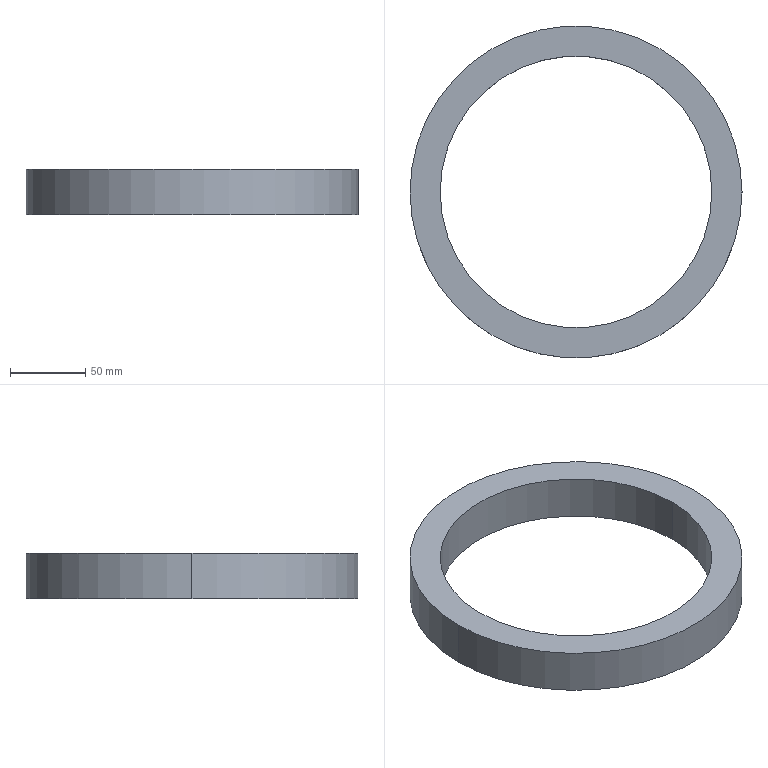Part | SolidWorks | features Extrusion 1 | 1 solid | 6 faces | box 220 x 220 x 30 mm | volume 376991 mm3 | cylinder 4 | plane 2 | commonest cylinder face diameters 180 x2 220 x2
STEP:
#1=CARTESIAN_POINT('',(-90.,0.,30.));
#2=VERTEX_POINT('',#1);
#3=CARTESIAN_POINT('',(90.,0.,30.));
#4=VERTEX_POINT('',#3);
#5=CARTESIAN_POINT('',(0.,0.,30.));
#6=DIRECTION('',(0.,0.,1.));
#7=DIRECTION('',(1.,0.,0.));
#8=AXIS2_PLACEMENT_3D('',#5,#6,#7);
#9=CIRCLE('',#8,90.);
#10=EDGE_CURVE('',#2,#4,#9,.T.);
#11=ORIENTED_EDGE('',*,*,#10,.T.);
#12=CARTESIAN_POINT('',(90.,0.,0.));
#13=VERTEX_POINT('',#12);
#14=CARTESIAN_POINT('',(90.,0.,30.));
#15=DIRECTION('',(0.,0.,-1.));
#16=VECTOR('',#15,1000.);
#17=LINE('',#14,#16);
#18=EDGE_CURVE('',#4,#13,#17,.T.);
#19=ORIENTED_EDGE('',*,*,#18,.T.);
#20=CARTESIAN_POINT('',(-90.,0.,0.));
#21=VERTEX_POINT('',#20);
#22=CARTESIAN_POINT('',(0.,0.,0.));
#23=DIRECTION('',(0.,0.,1.));
#24=DIRECTION('',(1.,0.,0.));
#25=AXIS2_PLACEMENT_3D('',#22,#23,#24);
#26=CIRCLE('',#25,90.);
#27=EDGE_CURVE('',#21,#13,#26,.T.);
#28=ORIENTED_EDGE('',*,*,#27,.F.);
#29=CARTESIAN_POINT('',(-90.,0.,30.));
#30=DIRECTION('',(0.,0.,-1.));
#31=VECTOR('',#30,1000.);
#32=LINE('',#29,#31);
#33=EDGE_CURVE('',#2,#21,#32,.T.);
#34=ORIENTED_EDGE('',*,*,#33,.F.);
#35=EDGE_LOOP('',(#11,#19,#28,#34));
#36=FACE_OUTER_BOUND('',#35,.T.);
#37=CARTESIAN_POINT('',(0.,0.,30.));
#38=DIRECTION('',(0.,0.,-1.));
#39=DIRECTION('',(-1.,0.,0.));
#40=AXIS2_PLACEMENT_3D('',#37,#38,#39);
#41=CYLINDRICAL_SURFACE('',#40,90.);
#42=ADVANCED_FACE('',(#36),#41,.F.);
#43=CARTESIAN_POINT('',(110.,0.,30.));
#44=VERTEX_POINT('',#43);
#45=CARTESIAN_POINT('',(-110.,0.,30.));
#46=VERTEX_POINT('',#45);
#47=CARTESIAN_POINT('',(0.,0.,30.));
#48=DIRECTION('',(0.,0.,1.));
#49=DIRECTION('',(1.,0.,0.));
#50=AXIS2_PLACEMENT_3D('',#47,#48,#49);
#51=CIRCLE('',#50,110.);
#52=EDGE_CURVE('',#44,#46,#51,.T.);
#53=ORIENTED_EDGE('',*,*,#52,.F.);
#54=CARTESIAN_POINT('',(110.,0.,0.));
#55=VERTEX_POINT('',#54);
#56=CARTESIAN_POINT('',(110.,0.,30.));
#57=DIRECTION('',(0.,0.,-1.));
#58=VECTOR('',#57,1000.);
#59=LINE('',#56,#58);
#60=EDGE_CURVE('',#44,#55,#59,.T.);
#61=ORIENTED_EDGE('',*,*,#60,.T.);
#62=CARTESIAN_POINT('',(-110.,0.,0.));
#63=VERTEX_POINT('',#62);
#64=CARTESIAN_POINT('',(0.,0.,0.));
#65=DIRECTION('',(0.,0.,1.));
#66=DIRECTION('',(1.,0.,0.));
#67=AXIS2_PLACEMENT_3D('',#64,#65,#66);
#68=CIRCLE('',#67,110.);
#69=EDGE_CURVE('',#55,#63,#68,.T.);
#70=ORIENTED_EDGE('',*,*,#69,.T.);
#71=CARTESIAN_POINT('',(-110.,0.,30.));
#72=DIRECTION('',(0.,0.,-1.));
#73=VECTOR('',#72,1000.);
#74=LINE('',#71,#73);
#75=EDGE_CURVE('',#46,#63,#74,.T.);
#76=ORIENTED_EDGE('',*,*,#75,.F.);
#77=EDGE_LOOP('',(#53,#61,#70,#76));
#78=FACE_OUTER_BOUND('',#77,.T.);
#79=CARTESIAN_POINT('',(0.,0.,30.));
#80=DIRECTION('',(0.,0.,-1.));
#81=DIRECTION('',(-1.,0.,0.));
#82=AXIS2_PLACEMENT_3D('',#79,#80,#81);
#83=CYLINDRICAL_SURFACE('',#82,110.);
#84=ADVANCED_FACE('',(#78),#83,.T.);
#85=CARTESIAN_POINT('',(0.,0.,30.));
#86=DIRECTION('',(0.,0.,1.));
#87=DIRECTION('',(1.,0.,0.));
#88=AXIS2_PLACEMENT_3D('',#85,#86,#87);
#89=CIRCLE('',#88,110.);
#90=EDGE_CURVE('',#46,#44,#89,.T.);
#91=ORIENTED_EDGE('',*,*,#90,.T.);
#92=ORIENTED_EDGE('',*,*,#52,.T.);
#93=EDGE_LOOP('',(#91,#92));
#94=FACE_OUTER_BOUND('',#93,.T.);
#95=ORIENTED_EDGE('',*,*,#10,.F.);
#96=CARTESIAN_POINT('',(0.,0.,30.));
#97=DIRECTION('',(0.,0.,1.));
#98=DIRECTION('',(1.,0.,0.));
#99=AXIS2_PLACEMENT_3D('',#96,#97,#98);
#100=CIRCLE('',#99,90.);
#101=EDGE_CURVE('',#4,#2,#100,.T.);
#102=ORIENTED_EDGE('',*,*,#101,.F.);
#103=EDGE_LOOP('',(#95,#102));
#104=FACE_BOUND('',#103,.T.);
#105=CARTESIAN_POINT('',(0.,0.,30.));
#106=DIRECTION('',(0.,0.,1.));
#107=DIRECTION('',(1.,0.,0.));
#108=AXIS2_PLACEMENT_3D('',#105,#106,#107);
#109=PLANE('',#108);
#110=ADVANCED_FACE('',(#94,#104),#109,.T.);
#111=CARTESIAN_POINT('',(0.,0.,0.));
#112=DIRECTION('',(0.,0.,1.));
#113=DIRECTION('',(1.,0.,0.));
#114=AXIS2_PLACEMENT_3D('',#111,#112,#113);
#115=CIRCLE('',#114,110.);
#116=EDGE_CURVE('',#63,#55,#115,.T.);
#117=ORIENTED_EDGE('',*,*,#116,.F.);
#118=ORIENTED_EDGE('',*,*,#69,.F.);
#119=EDGE_LOOP('',(#117,#118));
#120=FACE_OUTER_BOUND('',#119,.T.);
#121=ORIENTED_EDGE('',*,*,#27,.T.);
#122=CARTESIAN_POINT('',(0.,0.,0.));
#123=DIRECTION('',(0.,0.,1.));
#124=DIRECTION('',(1.,0.,0.));
#125=AXIS2_PLACEMENT_3D('',#122,#123,#124);
#126=CIRCLE('',#125,90.);
#127=EDGE_CURVE('',#13,#21,#126,.T.);
#128=ORIENTED_EDGE('',*,*,#127,.T.);
#129=EDGE_LOOP('',(#121,#128));
#130=FACE_BOUND('',#129,.T.);
#131=CARTESIAN_POINT('',(0.,0.,0.));
#132=DIRECTION('',(0.,0.,1.));
#133=DIRECTION('',(1.,0.,0.));
#134=AXIS2_PLACEMENT_3D('',#131,#132,#133);
#135=PLANE('',#134);
#136=ADVANCED_FACE('',(#120,#130),#135,.F.);
#137=ORIENTED_EDGE('',*,*,#60,.F.);
#138=ORIENTED_EDGE('',*,*,#90,.F.);
#139=ORIENTED_EDGE('',*,*,#75,.T.);
#140=ORIENTED_EDGE('',*,*,#116,.T.);
#141=EDGE_LOOP('',(#137,#138,#139,#140));
#142=FACE_OUTER_BOUND('',#141,.T.);
#143=CARTESIAN_POINT('',(0.,0.,30.));
#144=DIRECTION('',(0.,0.,-1.));
#145=DIRECTION('',(-1.,0.,0.));
#146=AXIS2_PLACEMENT_3D('',#143,#144,#145);
#147=CYLINDRICAL_SURFACE('',#146,110.);
#148=ADVANCED_FACE('',(#142),#147,.T.);
#149=ORIENTED_EDGE('',*,*,#18,.F.);
#150=ORIENTED_EDGE('',*,*,#101,.T.);
#151=ORIENTED_EDGE('',*,*,#33,.T.);
#152=ORIENTED_EDGE('',*,*,#127,.F.);
#153=EDGE_LOOP('',(#149,#150,#151,#152));
#154=FACE_OUTER_BOUND('',#153,.T.);
#155=CARTESIAN_POINT('',(0.,0.,30.));
#156=DIRECTION('',(0.,0.,-1.));
#157=DIRECTION('',(-1.,0.,0.));
#158=AXIS2_PLACEMENT_3D('',#155,#156,#157);
#159=CYLINDRICAL_SURFACE('',#158,90.);
#160=ADVANCED_FACE('',(#154),#159,.F.);
#161=CLOSED_SHELL('',(#42,#84,#110,#136,#148,#160));
#162=MANIFOLD_SOLID_BREP('',#161);
#163=CARTESIAN_POINT('',(0.,0.,0.));
#164=DIRECTION('',(0.,0.,1.));
#165=DIRECTION('',(1.,0.,0.));
#166=AXIS2_PLACEMENT_3D('',#163,#164,#165);
#167=(LENGTH_UNIT()NAMED_UNIT(*)SI_UNIT(.MILLI.,.METRE.));
#168=UNCERTAINTY_MEASURE_WITH_UNIT(LENGTH_MEASURE(0.00001),#167,'','');
#169=(NAMED_UNIT(*)PLANE_ANGLE_UNIT()SI_UNIT($,.RADIAN.));
#170=(NAMED_UNIT(*)SI_UNIT($,.STERADIAN.)SOLID_ANGLE_UNIT());
#171=(GEOMETRIC_REPRESENTATION_CONTEXT(3)GLOBAL_UNCERTAINTY_ASSIGNED_CONTEXT((#168))GLOBAL_UNIT_ASSIGNED_CONTEXT((#167,#169,#170))REPRESENTATION_CONTEXT('',''));
#172=ADVANCED_BREP_SHAPE_REPRESENTATION('',(#162,#166),#171);